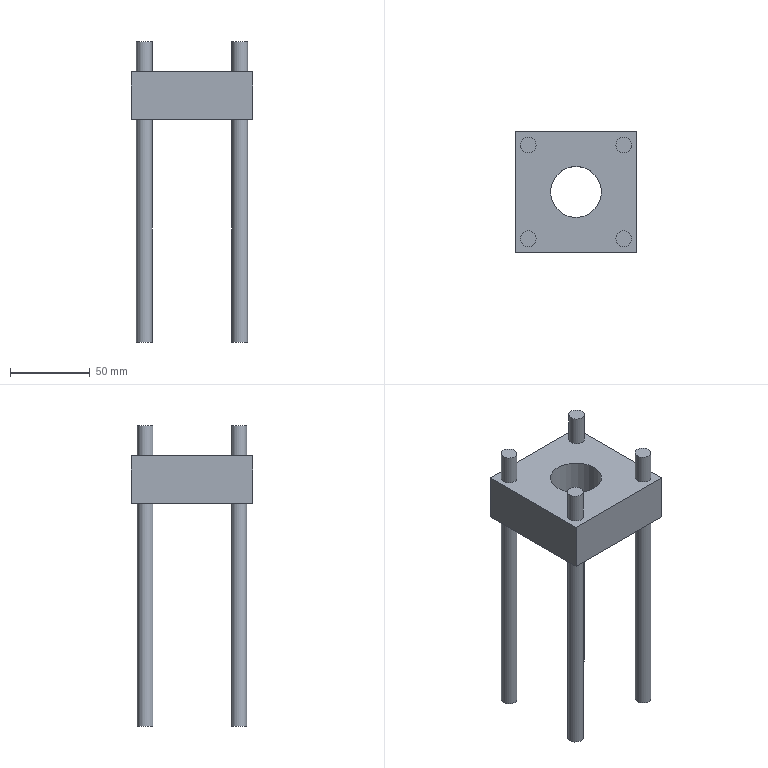Part | NX | features solid 2 | 1 solid | 25 faces | box 76 x 76 x 189 mm | volume 194032 mm3 | plane 15 | cylinder 10 | commonest cylinder face diameters 9.874 x8 18 x1 32 x1
STEP:
#1=CARTESIAN_POINT('',(6.,-117.,-165.));
#2=VERTEX_POINT('',#1);
#3=CARTESIAN_POINT('',(-3.,-117.,-165.));
#4=DIRECTION('',(0.,-1.,0.));
#5=DIRECTION('',(1.,0.,0.));
#6=AXIS2_PLACEMENT_3D('',#3,#4,#5);
#7=CIRCLE('',#6,9.);
#8=EDGE_CURVE('',#2,#2,#7,.T.);
#9=ORIENTED_EDGE('',*,*,#8,.T.);
#10=EDGE_LOOP('',(#9));
#11=FACE_BOUND('',#10,.T.);
#12=CARTESIAN_POINT('',(-38.,-117.,-150.));
#13=VERTEX_POINT('',#12);
#14=CARTESIAN_POINT('',(38.,-117.,-150.));
#15=VERTEX_POINT('',#14);
#16=CARTESIAN_POINT('',(-38.,-117.,-150.));
#17=DIRECTION('',(1.,0.,0.));
#18=VECTOR('',#17,1000.);
#19=LINE('',#16,#18);
#20=EDGE_CURVE('',#13,#15,#19,.T.);
#21=ORIENTED_EDGE('',*,*,#20,.T.);
#22=CARTESIAN_POINT('',(38.,-117.,-180.));
#23=VERTEX_POINT('',#22);
#24=CARTESIAN_POINT('',(38.,-117.,-180.));
#25=DIRECTION('',(0.,0.,1.));
#26=VECTOR('',#25,1000.);
#27=LINE('',#24,#26);
#28=EDGE_CURVE('',#23,#15,#27,.T.);
#29=ORIENTED_EDGE('',*,*,#28,.F.);
#30=CARTESIAN_POINT('',(-38.,-117.,-180.));
#31=VERTEX_POINT('',#30);
#32=CARTESIAN_POINT('',(-38.,-117.,-180.));
#33=DIRECTION('',(1.,0.,0.));
#34=VECTOR('',#33,1000.);
#35=LINE('',#32,#34);
#36=EDGE_CURVE('',#31,#23,#35,.T.);
#37=ORIENTED_EDGE('',*,*,#36,.F.);
#38=CARTESIAN_POINT('',(-38.,-117.,-180.));
#39=DIRECTION('',(0.,0.,1.));
#40=VECTOR('',#39,1000.);
#41=LINE('',#38,#40);
#42=EDGE_CURVE('',#31,#13,#41,.T.);
#43=ORIENTED_EDGE('',*,*,#42,.T.);
#44=EDGE_LOOP('',(#21,#29,#37,#43));
#45=FACE_BOUND('',#44,.T.);
#46=CARTESIAN_POINT('',(-38.,-117.,-180.));
#47=DIRECTION('',(0.,-1.,0.));
#48=DIRECTION('',(1.,0.,0.));
#49=AXIS2_PLACEMENT_3D('',#46,#47,#48);
#50=PLANE('',#49);
#51=ADVANCED_FACE('',(#11,#45),#50,.F.);
#52=CARTESIAN_POINT('',(-38.,-193.,-150.));
#53=VERTEX_POINT('',#52);
#54=CARTESIAN_POINT('',(-38.,-155.,-150.));
#55=DIRECTION('',(0.,-1.,0.));
#56=VECTOR('',#55,1000.);
#57=LINE('',#54,#56);
#58=EDGE_CURVE('',#13,#53,#57,.T.);
#59=ORIENTED_EDGE('',*,*,#58,.F.);
#60=ORIENTED_EDGE('',*,*,#42,.F.);
#61=CARTESIAN_POINT('',(-38.,-193.,-180.));
#62=VERTEX_POINT('',#61);
#63=CARTESIAN_POINT('',(-38.,-155.,-180.));
#64=DIRECTION('',(0.,1.,0.));
#65=VECTOR('',#64,1000.);
#66=LINE('',#63,#65);
#67=EDGE_CURVE('',#62,#31,#66,.T.);
#68=ORIENTED_EDGE('',*,*,#67,.F.);
#69=CARTESIAN_POINT('',(-38.,-193.,-180.));
#70=DIRECTION('',(0.,0.,1.));
#71=VECTOR('',#70,1000.);
#72=LINE('',#69,#71);
#73=EDGE_CURVE('',#62,#53,#72,.T.);
#74=ORIENTED_EDGE('',*,*,#73,.T.);
#75=EDGE_LOOP('',(#59,#60,#68,#74));
#76=FACE_BOUND('',#75,.T.);
#77=CARTESIAN_POINT('',(-38.,-155.,-180.));
#78=DIRECTION('',(-1.,0.,0.));
#79=DIRECTION('',(0.,-1.,0.));
#80=AXIS2_PLACEMENT_3D('',#77,#78,#79);
#81=PLANE('',#80);
#82=ADVANCED_FACE('',(#76),#81,.T.);
#83=CARTESIAN_POINT('',(38.,-193.,-150.));
#84=VERTEX_POINT('',#83);
#85=CARTESIAN_POINT('',(38.,-193.,-150.));
#86=DIRECTION('',(-1.,0.,0.));
#87=VECTOR('',#86,1000.);
#88=LINE('',#85,#87);
#89=EDGE_CURVE('',#84,#53,#88,.T.);
#90=ORIENTED_EDGE('',*,*,#89,.T.);
#91=ORIENTED_EDGE('',*,*,#73,.F.);
#92=CARTESIAN_POINT('',(38.,-193.,-180.));
#93=VERTEX_POINT('',#92);
#94=CARTESIAN_POINT('',(-38.,-193.,-180.));
#95=DIRECTION('',(1.,0.,0.));
#96=VECTOR('',#95,1000.);
#97=LINE('',#94,#96);
#98=EDGE_CURVE('',#62,#93,#97,.T.);
#99=ORIENTED_EDGE('',*,*,#98,.T.);
#100=CARTESIAN_POINT('',(38.,-193.,-180.));
#101=DIRECTION('',(0.,0.,1.));
#102=VECTOR('',#101,1000.);
#103=LINE('',#100,#102);
#104=EDGE_CURVE('',#93,#84,#103,.T.);
#105=ORIENTED_EDGE('',*,*,#104,.T.);
#106=EDGE_LOOP('',(#90,#91,#99,#105));
#107=FACE_BOUND('',#106,.T.);
#108=CARTESIAN_POINT('',(38.,-193.,-180.));
#109=DIRECTION('',(0.,1.,0.));
#110=DIRECTION('',(0.,0.,-1.));
#111=AXIS2_PLACEMENT_3D('',#108,#109,#110);
#112=PLANE('',#111);
#113=ADVANCED_FACE('',(#107),#112,.F.);
#114=CARTESIAN_POINT('',(38.,-155.,-150.));
#115=DIRECTION('',(0.,1.,0.));
#116=VECTOR('',#115,1000.);
#117=LINE('',#114,#116);
#118=EDGE_CURVE('',#84,#15,#117,.T.);
#119=ORIENTED_EDGE('',*,*,#118,.F.);
#120=ORIENTED_EDGE('',*,*,#104,.F.);
#121=CARTESIAN_POINT('',(38.,-155.,-180.));
#122=DIRECTION('',(0.,-1.,0.));
#123=VECTOR('',#122,1000.);
#124=LINE('',#121,#123);
#125=EDGE_CURVE('',#23,#93,#124,.T.);
#126=ORIENTED_EDGE('',*,*,#125,.F.);
#127=ORIENTED_EDGE('',*,*,#28,.T.);
#128=EDGE_LOOP('',(#119,#120,#126,#127));
#129=FACE_BOUND('',#128,.T.);
#130=CARTESIAN_POINT('',(38.,-155.,-180.));
#131=DIRECTION('',(1.,0.,0.));
#132=DIRECTION('',(0.,1.,0.));
#133=AXIS2_PLACEMENT_3D('',#130,#131,#132);
#134=PLANE('',#133);
#135=ADVANCED_FACE('',(#129),#134,.T.);
#136=CARTESIAN_POINT('',(-16.,-155.,-180.));
#137=VERTEX_POINT('',#136);
#138=CARTESIAN_POINT('',(0.,-155.,-180.));
#139=DIRECTION('',(0.,0.,1.));
#140=DIRECTION('',(-1.,0.,0.));
#141=AXIS2_PLACEMENT_3D('',#138,#139,#140);
#142=CIRCLE('',#141,16.);
#143=EDGE_CURVE('',#137,#137,#142,.T.);
#144=ORIENTED_EDGE('',*,*,#143,.T.);
#145=EDGE_LOOP('',(#144));
#146=FACE_BOUND('',#145,.T.);
#147=CARTESIAN_POINT('',(-34.937,-125.594,-180.));
#148=VERTEX_POINT('',#147);
#149=CARTESIAN_POINT('',(-30.,-125.594,-180.));
#150=DIRECTION('',(0.,0.,1.));
#151=DIRECTION('',(-1.,0.,0.));
#152=AXIS2_PLACEMENT_3D('',#149,#150,#151);
#153=CIRCLE('',#152,4.937);
#154=EDGE_CURVE('',#148,#148,#153,.T.);
#155=ORIENTED_EDGE('',*,*,#154,.T.);
#156=EDGE_LOOP('',(#155));
#157=FACE_BOUND('',#156,.T.);
#158=CARTESIAN_POINT('',(-34.937,-184.406,-180.));
#159=VERTEX_POINT('',#158);
#160=CARTESIAN_POINT('',(-30.,-184.406,-180.));
#161=DIRECTION('',(0.,0.,-1.));
#162=DIRECTION('',(-1.,0.,0.));
#163=AXIS2_PLACEMENT_3D('',#160,#161,#162);
#164=CIRCLE('',#163,4.937);
#165=EDGE_CURVE('',#159,#159,#164,.T.);
#166=ORIENTED_EDGE('',*,*,#165,.F.);
#167=EDGE_LOOP('',(#166));
#168=FACE_BOUND('',#167,.T.);
#169=ORIENTED_EDGE('',*,*,#36,.T.);
#170=ORIENTED_EDGE('',*,*,#125,.T.);
#171=ORIENTED_EDGE('',*,*,#98,.F.);
#172=ORIENTED_EDGE('',*,*,#67,.T.);
#173=EDGE_LOOP('',(#169,#170,#171,#172));
#174=FACE_BOUND('',#173,.T.);
#175=CARTESIAN_POINT('',(25.063,-184.406,-180.));
#176=VERTEX_POINT('',#175);
#177=CARTESIAN_POINT('',(30.,-184.406,-180.));
#178=DIRECTION('',(0.,0.,1.));
#179=DIRECTION('',(-1.,0.,0.));
#180=AXIS2_PLACEMENT_3D('',#177,#178,#179);
#181=CIRCLE('',#180,4.937);
#182=EDGE_CURVE('',#176,#176,#181,.T.);
#183=ORIENTED_EDGE('',*,*,#182,.T.);
#184=EDGE_LOOP('',(#183));
#185=FACE_BOUND('',#184,.T.);
#186=CARTESIAN_POINT('',(34.937,-125.594,-180.));
#187=VERTEX_POINT('',#186);
#188=CARTESIAN_POINT('',(30.,-125.594,-180.));
#189=DIRECTION('',(0.,0.,-1.));
#190=DIRECTION('',(1.,0.,0.));
#191=AXIS2_PLACEMENT_3D('',#188,#189,#190);
#192=CIRCLE('',#191,4.937);
#193=EDGE_CURVE('',#187,#187,#192,.T.);
#194=ORIENTED_EDGE('',*,*,#193,.F.);
#195=EDGE_LOOP('',(#194));
#196=FACE_BOUND('',#195,.T.);
#197=CARTESIAN_POINT('',(38.,-117.,-180.));
#198=DIRECTION('',(0.,0.,1.));
#199=DIRECTION('',(-1.,0.,0.));
#200=AXIS2_PLACEMENT_3D('',#197,#198,#199);
#201=PLANE('',#200);
#202=ADVANCED_FACE('',(#146,#157,#168,#174,#185,#196),#201,.F.);
#203=CARTESIAN_POINT('',(-16.,-155.,-150.));
#204=VERTEX_POINT('',#203);
#205=CARTESIAN_POINT('',(0.,-155.,-150.));
#206=DIRECTION('',(0.,0.,1.));
#207=DIRECTION('',(-1.,0.,0.));
#208=AXIS2_PLACEMENT_3D('',#205,#206,#207);
#209=CIRCLE('',#208,16.);
#210=EDGE_CURVE('',#204,#204,#209,.T.);
#211=ORIENTED_EDGE('',*,*,#210,.F.);
#212=EDGE_LOOP('',(#211));
#213=FACE_BOUND('',#212,.T.);
#214=CARTESIAN_POINT('',(-34.937,-125.594,-150.));
#215=VERTEX_POINT('',#214);
#216=CARTESIAN_POINT('',(-30.,-125.594,-150.));
#217=DIRECTION('',(0.,0.,1.));
#218=DIRECTION('',(-1.,0.,0.));
#219=AXIS2_PLACEMENT_3D('',#216,#217,#218);
#220=CIRCLE('',#219,4.937);
#221=EDGE_CURVE('',#215,#215,#220,.T.);
#222=ORIENTED_EDGE('',*,*,#221,.F.);
#223=EDGE_LOOP('',(#222));
#224=FACE_BOUND('',#223,.T.);
#225=CARTESIAN_POINT('',(-34.937,-184.406,-150.));
#226=VERTEX_POINT('',#225);
#227=CARTESIAN_POINT('',(-30.,-184.406,-150.));
#228=DIRECTION('',(0.,0.,1.));
#229=DIRECTION('',(-1.,0.,0.));
#230=AXIS2_PLACEMENT_3D('',#227,#228,#229);
#231=CIRCLE('',#230,4.937);
#232=EDGE_CURVE('',#226,#226,#231,.F.);
#233=ORIENTED_EDGE('',*,*,#232,.T.);
#234=EDGE_LOOP('',(#233));
#235=FACE_BOUND('',#234,.T.);
#236=ORIENTED_EDGE('',*,*,#118,.T.);
#237=ORIENTED_EDGE('',*,*,#20,.F.);
#238=ORIENTED_EDGE('',*,*,#58,.T.);
#239=ORIENTED_EDGE('',*,*,#89,.F.);
#240=EDGE_LOOP('',(#236,#237,#238,#239));
#241=FACE_BOUND('',#240,.T.);
#242=CARTESIAN_POINT('',(34.937,-184.406,-150.));
#243=VERTEX_POINT('',#242);
#244=CARTESIAN_POINT('',(30.,-184.406,-150.));
#245=DIRECTION('',(0.,0.,1.));
#246=DIRECTION('',(1.,0.,0.));
#247=AXIS2_PLACEMENT_3D('',#244,#245,#246);
#248=CIRCLE('',#247,4.937);
#249=EDGE_CURVE('',#243,#243,#248,.T.);
#250=ORIENTED_EDGE('',*,*,#249,.F.);
#251=EDGE_LOOP('',(#250));
#252=FACE_BOUND('',#251,.T.);
#253=CARTESIAN_POINT('',(25.063,-125.594,-150.));
#254=VERTEX_POINT('',#253);
#255=CARTESIAN_POINT('',(30.,-125.594,-150.));
#256=DIRECTION('',(0.,0.,1.));
#257=DIRECTION('',(-1.,0.,0.));
#258=AXIS2_PLACEMENT_3D('',#255,#256,#257);
#259=CIRCLE('',#258,4.937);
#260=EDGE_CURVE('',#254,#254,#259,.F.);
#261=ORIENTED_EDGE('',*,*,#260,.T.);
#262=EDGE_LOOP('',(#261));
#263=FACE_BOUND('',#262,.T.);
#264=CARTESIAN_POINT('',(38.,-117.,-150.));
#265=DIRECTION('',(0.,0.,1.));
#266=DIRECTION('',(-1.,0.,0.));
#267=AXIS2_PLACEMENT_3D('',#264,#265,#266);
#268=PLANE('',#267);
#269=ADVANCED_FACE('',(#213,#224,#235,#241,#252,#263),#268,.T.);
#270=CARTESIAN_POINT('',(-34.937,-184.406,-131.));
#271=VERTEX_POINT('',#270);
#272=CARTESIAN_POINT('',(-30.,-184.406,-131.));
#273=DIRECTION('',(0.,0.,-1.));
#274=DIRECTION('',(-1.,0.,0.));
#275=AXIS2_PLACEMENT_3D('',#272,#273,#274);
#276=CIRCLE('',#275,4.937);
#277=EDGE_CURVE('',#271,#271,#276,.T.);
#278=ORIENTED_EDGE('',*,*,#277,.F.);
#279=EDGE_LOOP('',(#278));
#280=FACE_BOUND('',#279,.T.);
#281=CARTESIAN_POINT('',(-30.,-184.406,-131.));
#282=DIRECTION('',(0.,0.,-1.));
#283=DIRECTION('',(1.,0.,0.));
#284=AXIS2_PLACEMENT_3D('',#281,#282,#283);
#285=PLANE('',#284);
#286=ADVANCED_FACE('',(#280),#285,.F.);
#287=ORIENTED_EDGE('',*,*,#232,.F.);
#288=EDGE_LOOP('',(#287));
#289=FACE_BOUND('',#288,.T.);
#290=ORIENTED_EDGE('',*,*,#277,.T.);
#291=EDGE_LOOP('',(#290));
#292=FACE_BOUND('',#291,.T.);
#293=CARTESIAN_POINT('',(-30.,-184.406,-320.));
#294=DIRECTION('',(0.,0.,1.));
#295=DIRECTION('',(-1.,0.,0.));
#296=AXIS2_PLACEMENT_3D('',#293,#294,#295);
#297=CYLINDRICAL_SURFACE('',#296,4.937);
#298=ADVANCED_FACE('',(#289,#292),#297,.T.);
#299=CARTESIAN_POINT('',(-34.937,-184.406,-320.));
#300=VERTEX_POINT('',#299);
#301=CARTESIAN_POINT('',(-30.,-184.406,-320.));
#302=DIRECTION('',(0.,0.,-1.));
#303=DIRECTION('',(-1.,0.,0.));
#304=AXIS2_PLACEMENT_3D('',#301,#302,#303);
#305=CIRCLE('',#304,4.937);
#306=EDGE_CURVE('',#300,#300,#305,.T.);
#307=ORIENTED_EDGE('',*,*,#306,.F.);
#308=EDGE_LOOP('',(#307));
#309=FACE_BOUND('',#308,.T.);
#310=ORIENTED_EDGE('',*,*,#165,.T.);
#311=EDGE_LOOP('',(#310));
#312=FACE_BOUND('',#311,.T.);
#313=CARTESIAN_POINT('',(-30.,-184.406,-320.));
#314=DIRECTION('',(0.,0.,1.));
#315=DIRECTION('',(-1.,0.,0.));
#316=AXIS2_PLACEMENT_3D('',#313,#314,#315);
#317=CYLINDRICAL_SURFACE('',#316,4.937);
#318=ADVANCED_FACE('',(#309,#312),#317,.T.);
#319=ORIENTED_EDGE('',*,*,#306,.T.);
#320=EDGE_LOOP('',(#319));
#321=FACE_BOUND('',#320,.T.);
#322=CARTESIAN_POINT('',(-30.,-184.406,-320.));
#323=DIRECTION('',(0.,0.,-1.));
#324=DIRECTION('',(1.,0.,0.));
#325=AXIS2_PLACEMENT_3D('',#322,#323,#324);
#326=PLANE('',#325);
#327=ADVANCED_FACE('',(#321),#326,.T.);
#328=CARTESIAN_POINT('',(34.937,-184.406,-131.));
#329=VERTEX_POINT('',#328);
#330=CARTESIAN_POINT('',(30.,-184.406,-131.));
#331=DIRECTION('',(0.,0.,1.));
#332=DIRECTION('',(1.,0.,0.));
#333=AXIS2_PLACEMENT_3D('',#330,#331,#332);
#334=CIRCLE('',#333,4.937);
#335=EDGE_CURVE('',#329,#329,#334,.T.);
#336=ORIENTED_EDGE('',*,*,#335,.T.);
#337=EDGE_LOOP('',(#336));
#338=FACE_BOUND('',#337,.T.);
#339=CARTESIAN_POINT('',(30.,-184.406,-131.));
#340=DIRECTION('',(0.,0.,1.));
#341=DIRECTION('',(-1.,0.,0.));
#342=AXIS2_PLACEMENT_3D('',#339,#340,#341);
#343=PLANE('',#342);
#344=ADVANCED_FACE('',(#338),#343,.T.);
#345=ORIENTED_EDGE('',*,*,#249,.T.);
#346=EDGE_LOOP('',(#345));
#347=FACE_BOUND('',#346,.T.);
#348=ORIENTED_EDGE('',*,*,#335,.F.);
#349=EDGE_LOOP('',(#348));
#350=FACE_BOUND('',#349,.T.);
#351=CARTESIAN_POINT('',(30.,-184.406,-320.));
#352=DIRECTION('',(0.,0.,1.));
#353=DIRECTION('',(-1.,0.,0.));
#354=AXIS2_PLACEMENT_3D('',#351,#352,#353);
#355=CYLINDRICAL_SURFACE('',#354,4.937);
#356=ADVANCED_FACE('',(#347,#350),#355,.T.);
#357=CARTESIAN_POINT('',(34.937,-184.406,-320.));
#358=VERTEX_POINT('',#357);
#359=CARTESIAN_POINT('',(30.,-184.406,-320.));
#360=DIRECTION('',(0.,0.,1.));
#361=DIRECTION('',(1.,0.,0.));
#362=AXIS2_PLACEMENT_3D('',#359,#360,#361);
#363=CIRCLE('',#362,4.937);
#364=EDGE_CURVE('',#358,#358,#363,.T.);
#365=ORIENTED_EDGE('',*,*,#364,.T.);
#366=EDGE_LOOP('',(#365));
#367=FACE_BOUND('',#366,.T.);
#368=ORIENTED_EDGE('',*,*,#182,.F.);
#369=EDGE_LOOP('',(#368));
#370=FACE_BOUND('',#369,.T.);
#371=CARTESIAN_POINT('',(30.,-184.406,-320.));
#372=DIRECTION('',(0.,0.,1.));
#373=DIRECTION('',(-1.,0.,0.));
#374=AXIS2_PLACEMENT_3D('',#371,#372,#373);
#375=CYLINDRICAL_SURFACE('',#374,4.937);
#376=ADVANCED_FACE('',(#367,#370),#375,.T.);
#377=ORIENTED_EDGE('',*,*,#364,.F.);
#378=EDGE_LOOP('',(#377));
#379=FACE_BOUND('',#378,.T.);
#380=CARTESIAN_POINT('',(30.,-184.406,-320.));
#381=DIRECTION('',(0.,0.,1.));
#382=DIRECTION('',(-1.,0.,0.));
#383=AXIS2_PLACEMENT_3D('',#380,#381,#382);
#384=PLANE('',#383);
#385=ADVANCED_FACE('',(#379),#384,.F.);
#386=CARTESIAN_POINT('',(34.937,-125.594,-131.));
#387=VERTEX_POINT('',#386);
#388=CARTESIAN_POINT('',(30.,-125.594,-131.));
#389=DIRECTION('',(0.,0.,-1.));
#390=DIRECTION('',(1.,0.,0.));
#391=AXIS2_PLACEMENT_3D('',#388,#389,#390);
#392=CIRCLE('',#391,4.937);
#393=EDGE_CURVE('',#387,#387,#392,.T.);
#394=ORIENTED_EDGE('',*,*,#393,.F.);
#395=EDGE_LOOP('',(#394));
#396=FACE_BOUND('',#395,.T.);
#397=CARTESIAN_POINT('',(30.,-125.594,-131.));
#398=DIRECTION('',(0.,0.,-1.));
#399=DIRECTION('',(1.,0.,0.));
#400=AXIS2_PLACEMENT_3D('',#397,#398,#399);
#401=PLANE('',#400);
#402=ADVANCED_FACE('',(#396),#401,.F.);
#403=ORIENTED_EDGE('',*,*,#260,.F.);
#404=EDGE_LOOP('',(#403));
#405=FACE_BOUND('',#404,.T.);
#406=ORIENTED_EDGE('',*,*,#393,.T.);
#407=EDGE_LOOP('',(#406));
#408=FACE_BOUND('',#407,.T.);
#409=CARTESIAN_POINT('',(30.,-125.594,-320.));
#410=DIRECTION('',(0.,0.,1.));
#411=DIRECTION('',(-1.,0.,0.));
#412=AXIS2_PLACEMENT_3D('',#409,#410,#411);
#413=CYLINDRICAL_SURFACE('',#412,4.937);
#414=ADVANCED_FACE('',(#405,#408),#413,.T.);
#415=CARTESIAN_POINT('',(34.937,-125.594,-320.));
#416=VERTEX_POINT('',#415);
#417=CARTESIAN_POINT('',(30.,-125.594,-320.));
#418=DIRECTION('',(0.,0.,-1.));
#419=DIRECTION('',(1.,0.,0.));
#420=AXIS2_PLACEMENT_3D('',#417,#418,#419);
#421=CIRCLE('',#420,4.937);
#422=EDGE_CURVE('',#416,#416,#421,.T.);
#423=ORIENTED_EDGE('',*,*,#422,.F.);
#424=EDGE_LOOP('',(#423));
#425=FACE_BOUND('',#424,.T.);
#426=ORIENTED_EDGE('',*,*,#193,.T.);
#427=EDGE_LOOP('',(#426));
#428=FACE_BOUND('',#427,.T.);
#429=CARTESIAN_POINT('',(30.,-125.594,-320.));
#430=DIRECTION('',(0.,0.,1.));
#431=DIRECTION('',(-1.,0.,0.));
#432=AXIS2_PLACEMENT_3D('',#429,#430,#431);
#433=CYLINDRICAL_SURFACE('',#432,4.937);
#434=ADVANCED_FACE('',(#425,#428),#433,.T.);
#435=ORIENTED_EDGE('',*,*,#422,.T.);
#436=EDGE_LOOP('',(#435));
#437=FACE_BOUND('',#436,.T.);
#438=CARTESIAN_POINT('',(30.,-125.594,-320.));
#439=DIRECTION('',(0.,0.,-1.));
#440=DIRECTION('',(1.,0.,0.));
#441=AXIS2_PLACEMENT_3D('',#438,#439,#440);
#442=PLANE('',#441);
#443=ADVANCED_FACE('',(#437),#442,.T.);
#444=CARTESIAN_POINT('',(-34.937,-125.594,-131.));
#445=VERTEX_POINT('',#444);
#446=CARTESIAN_POINT('',(-30.,-125.594,-131.));
#447=DIRECTION('',(0.,0.,1.));
#448=DIRECTION('',(-1.,0.,0.));
#449=AXIS2_PLACEMENT_3D('',#446,#447,#448);
#450=CIRCLE('',#449,4.937);
#451=EDGE_CURVE('',#445,#445,#450,.T.);
#452=ORIENTED_EDGE('',*,*,#451,.T.);
#453=EDGE_LOOP('',(#452));
#454=FACE_BOUND('',#453,.T.);
#455=CARTESIAN_POINT('',(-30.,-125.594,-131.));
#456=DIRECTION('',(0.,0.,1.));
#457=DIRECTION('',(-1.,0.,0.));
#458=AXIS2_PLACEMENT_3D('',#455,#456,#457);
#459=PLANE('',#458);
#460=ADVANCED_FACE('',(#454),#459,.T.);
#461=ORIENTED_EDGE('',*,*,#221,.T.);
#462=EDGE_LOOP('',(#461));
#463=FACE_BOUND('',#462,.T.);
#464=ORIENTED_EDGE('',*,*,#451,.F.);
#465=EDGE_LOOP('',(#464));
#466=FACE_BOUND('',#465,.T.);
#467=CARTESIAN_POINT('',(-30.,-125.594,-320.));
#468=DIRECTION('',(0.,0.,1.));
#469=DIRECTION('',(-1.,0.,0.));
#470=AXIS2_PLACEMENT_3D('',#467,#468,#469);
#471=CYLINDRICAL_SURFACE('',#470,4.937);
#472=ADVANCED_FACE('',(#463,#466),#471,.T.);
#473=CARTESIAN_POINT('',(-34.937,-125.594,-320.));
#474=VERTEX_POINT('',#473);
#475=CARTESIAN_POINT('',(-30.,-125.594,-320.));
#476=DIRECTION('',(0.,0.,1.));
#477=DIRECTION('',(-1.,0.,0.));
#478=AXIS2_PLACEMENT_3D('',#475,#476,#477);
#479=CIRCLE('',#478,4.937);
#480=EDGE_CURVE('',#474,#474,#479,.T.);
#481=ORIENTED_EDGE('',*,*,#480,.T.);
#482=EDGE_LOOP('',(#481));
#483=FACE_BOUND('',#482,.T.);
#484=ORIENTED_EDGE('',*,*,#154,.F.);
#485=EDGE_LOOP('',(#484));
#486=FACE_BOUND('',#485,.T.);
#487=CARTESIAN_POINT('',(-30.,-125.594,-320.));
#488=DIRECTION('',(0.,0.,1.));
#489=DIRECTION('',(-1.,0.,0.));
#490=AXIS2_PLACEMENT_3D('',#487,#488,#489);
#491=CYLINDRICAL_SURFACE('',#490,4.937);
#492=ADVANCED_FACE('',(#483,#486),#491,.T.);
#493=ORIENTED_EDGE('',*,*,#480,.F.);
#494=EDGE_LOOP('',(#493));
#495=FACE_BOUND('',#494,.T.);
#496=CARTESIAN_POINT('',(-30.,-125.594,-320.));
#497=DIRECTION('',(0.,0.,1.));
#498=DIRECTION('',(-1.,0.,0.));
#499=AXIS2_PLACEMENT_3D('',#496,#497,#498);
#500=PLANE('',#499);
#501=ADVANCED_FACE('',(#495),#500,.F.);
#502=ORIENTED_EDGE('',*,*,#210,.T.);
#503=EDGE_LOOP('',(#502));
#504=FACE_BOUND('',#503,.T.);
#505=ORIENTED_EDGE('',*,*,#143,.F.);
#506=EDGE_LOOP('',(#505));
#507=FACE_BOUND('',#506,.T.);
#508=CARTESIAN_POINT('',(0.,-155.,-283.));
#509=DIRECTION('',(0.,0.,1.));
#510=DIRECTION('',(-1.,0.,0.));
#511=AXIS2_PLACEMENT_3D('',#508,#509,#510);
#512=CYLINDRICAL_SURFACE('',#511,16.);
#513=ADVANCED_FACE('',(#504,#507),#512,.F.);
#514=CARTESIAN_POINT('',(6.,-132.,-165.));
#515=VERTEX_POINT('',#514);
#516=CARTESIAN_POINT('',(-3.,-132.,-165.));
#517=DIRECTION('',(0.,-1.,0.));
#518=DIRECTION('',(1.,0.,0.));
#519=AXIS2_PLACEMENT_3D('',#516,#517,#518);
#520=CIRCLE('',#519,9.);
#521=EDGE_CURVE('',#515,#515,#520,.T.);
#522=ORIENTED_EDGE('',*,*,#521,.F.);
#523=EDGE_LOOP('',(#522));
#524=FACE_BOUND('',#523,.T.);
#525=CARTESIAN_POINT('',(-3.,-132.,-165.));
#526=DIRECTION('',(0.,-1.,0.));
#527=DIRECTION('',(1.,0.,0.));
#528=AXIS2_PLACEMENT_3D('',#525,#526,#527);
#529=PLANE('',#528);
#530=ADVANCED_FACE('',(#524),#529,.F.);
#531=ORIENTED_EDGE('',*,*,#521,.T.);
#532=EDGE_LOOP('',(#531));
#533=FACE_BOUND('',#532,.T.);
#534=ORIENTED_EDGE('',*,*,#8,.F.);
#535=EDGE_LOOP('',(#534));
#536=FACE_BOUND('',#535,.T.);
#537=CARTESIAN_POINT('',(-3.,-117.,-165.));
#538=DIRECTION('',(0.,-1.,0.));
#539=DIRECTION('',(1.,0.,0.));
#540=AXIS2_PLACEMENT_3D('',#537,#538,#539);
#541=CYLINDRICAL_SURFACE('',#540,9.);
#542=ADVANCED_FACE('',(#533,#536),#541,.F.);
#543=CLOSED_SHELL('',(#51,#82,#113,#135,#202,#269,#286,#298,#318,#327,#344,#356,#376,#385,#402,#414,#434,#443,#460,#472,#492,#501,#513,#530,#542));
#544=MANIFOLD_SOLID_BREP('',#543);
#545=(LENGTH_UNIT()NAMED_UNIT(*)SI_UNIT(.MILLI.,.METRE.));
#546=UNCERTAINTY_MEASURE_WITH_UNIT(LENGTH_MEASURE(0.00001),#545,'','');
#547=(NAMED_UNIT(*)PLANE_ANGLE_UNIT()SI_UNIT($,.RADIAN.));
#548=(NAMED_UNIT(*)SI_UNIT($,.STERADIAN.)SOLID_ANGLE_UNIT());
#549=(GEOMETRIC_REPRESENTATION_CONTEXT(3)GLOBAL_UNCERTAINTY_ASSIGNED_CONTEXT((#546))GLOBAL_UNIT_ASSIGNED_CONTEXT((#545,#547,#548))REPRESENTATION_CONTEXT('',''));
#550=ADVANCED_BREP_SHAPE_REPRESENTATION('',(#544),#549);